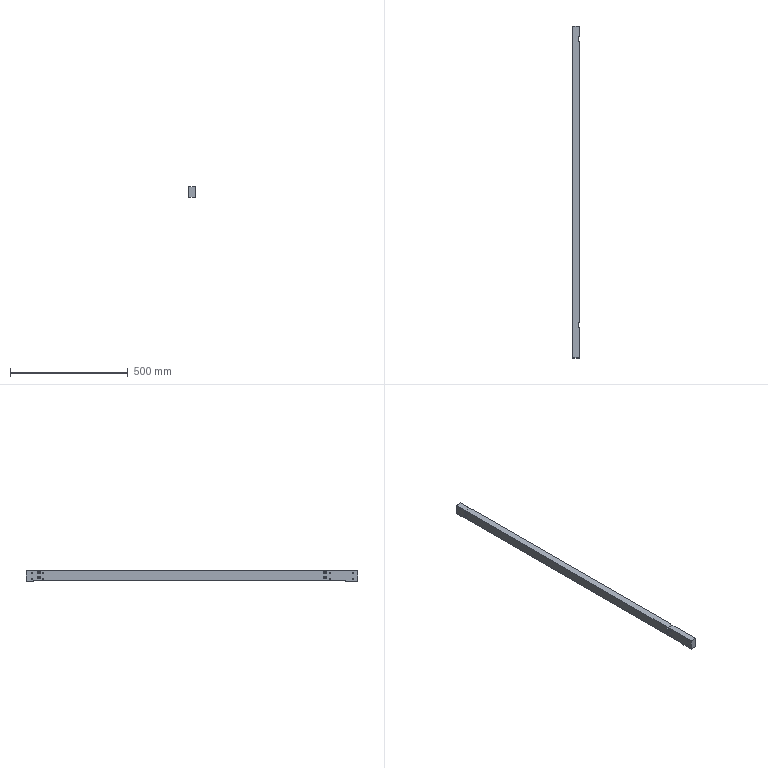Part | SolidWorks | features BaseBody 1 | 1 solid | 150 faces | box 27 x 1408 x 43 mm | volume 1477321 mm3 | cylinder 72 | cone 56 | plane 22 | commonest cylinder face diameters 3.3 x40 5 x16 6.6 x8 11 x8